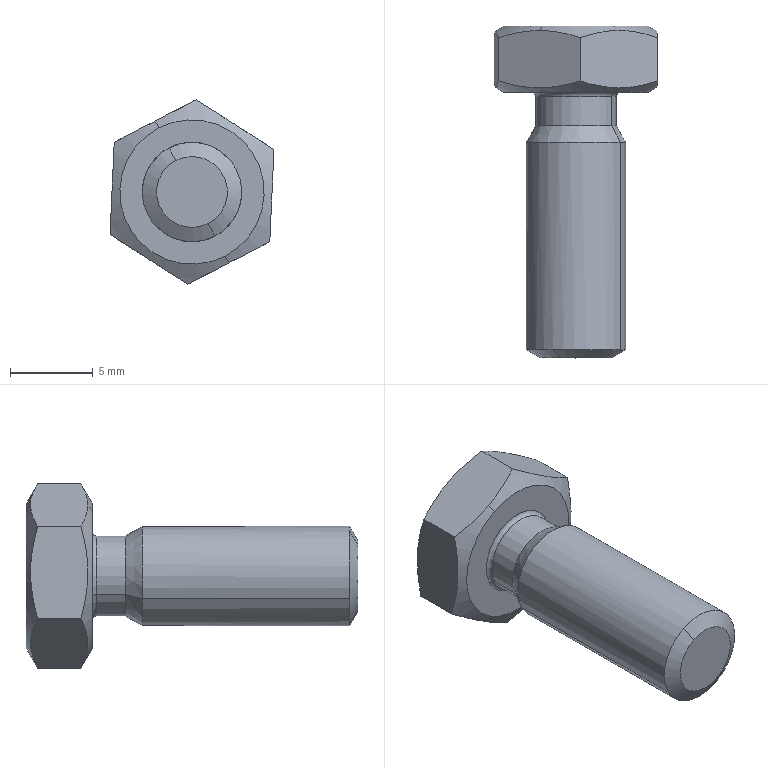Part | STEP file | Cut-Revolve 2-12 | 1 solid | 57 faces | box 9.884 x 20 x 11.12 mm | volume 653.571 mm3 | plane 41 | cone 8 | cylinder 6 | torus 2 | commonest cylinder face diameters 4.845 x2 6 x2 8.7 x2